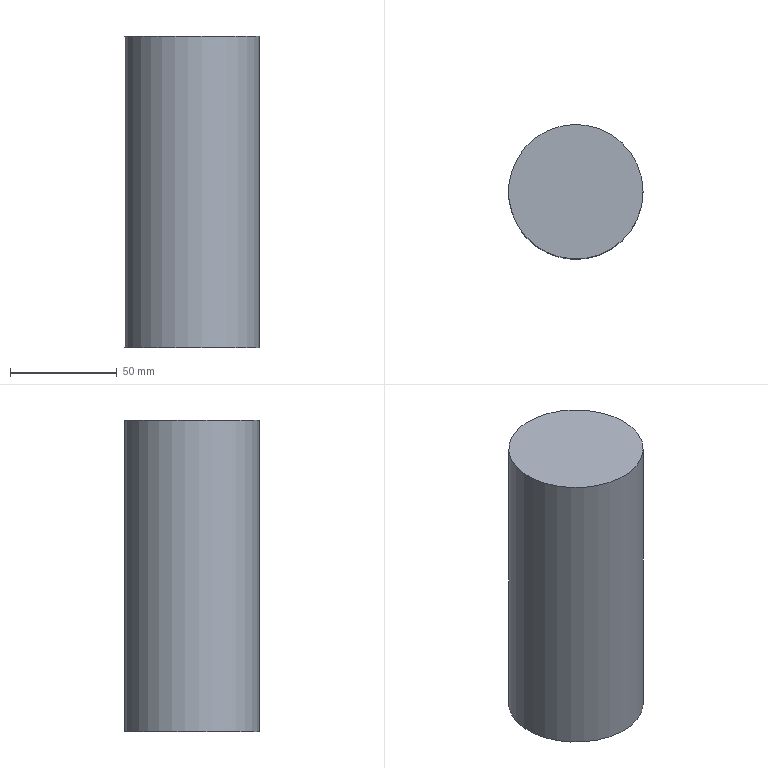Part | NX | features solid 2 | 1 solid | 3 faces | box 63 x 63 x 146 mm | volume 455118 mm3 | plane 2 | cylinder 1 | commonest cylinder face diameters 63 x1
STEP:
#1=CARTESIAN_POINT('',(31.5,-440.,-346.));
#2=VERTEX_POINT('',#1);
#3=CARTESIAN_POINT('',(0.,-440.,-346.));
#4=DIRECTION('',(0.,0.,1.));
#5=DIRECTION('',(1.,0.,0.));
#6=AXIS2_PLACEMENT_3D('',#3,#4,#5);
#7=CIRCLE('',#6,31.5);
#8=EDGE_CURVE('',#2,#2,#7,.T.);
#9=ORIENTED_EDGE('',*,*,#8,.T.);
#10=EDGE_LOOP('',(#9));
#11=FACE_BOUND('',#10,.T.);
#12=CARTESIAN_POINT('',(31.5,-440.,-200.));
#13=VERTEX_POINT('',#12);
#14=CARTESIAN_POINT('',(0.,-440.,-200.));
#15=DIRECTION('',(0.,0.,1.));
#16=DIRECTION('',(1.,0.,0.));
#17=AXIS2_PLACEMENT_3D('',#14,#15,#16);
#18=CIRCLE('',#17,31.5);
#19=EDGE_CURVE('',#13,#13,#18,.T.);
#20=ORIENTED_EDGE('',*,*,#19,.F.);
#21=EDGE_LOOP('',(#20));
#22=FACE_BOUND('',#21,.T.);
#23=CARTESIAN_POINT('',(0.,-440.,-476.));
#24=DIRECTION('',(0.,0.,1.));
#25=DIRECTION('',(-1.,0.,0.));
#26=AXIS2_PLACEMENT_3D('',#23,#24,#25);
#27=CYLINDRICAL_SURFACE('',#26,31.5);
#28=ADVANCED_FACE('',(#11,#22),#27,.T.);
#29=ORIENTED_EDGE('',*,*,#8,.F.);
#30=EDGE_LOOP('',(#29));
#31=FACE_BOUND('',#30,.T.);
#32=CARTESIAN_POINT('',(-35.,-475.,-346.));
#33=DIRECTION('',(0.,0.,-1.));
#34=DIRECTION('',(1.,0.,0.));
#35=AXIS2_PLACEMENT_3D('',#32,#33,#34);
#36=PLANE('',#35);
#37=ADVANCED_FACE('',(#31),#36,.T.);
#38=ORIENTED_EDGE('',*,*,#19,.T.);
#39=EDGE_LOOP('',(#38));
#40=FACE_BOUND('',#39,.T.);
#41=CARTESIAN_POINT('',(0.,-440.,-200.));
#42=DIRECTION('',(0.,0.,-1.));
#43=DIRECTION('',(1.,0.,0.));
#44=AXIS2_PLACEMENT_3D('',#41,#42,#43);
#45=PLANE('',#44);
#46=ADVANCED_FACE('',(#40),#45,.F.);
#47=CLOSED_SHELL('',(#28,#37,#46));
#48=MANIFOLD_SOLID_BREP('',#47);
#49=(LENGTH_UNIT()NAMED_UNIT(*)SI_UNIT(.MILLI.,.METRE.));
#50=UNCERTAINTY_MEASURE_WITH_UNIT(LENGTH_MEASURE(0.00001),#49,'','');
#51=(NAMED_UNIT(*)PLANE_ANGLE_UNIT()SI_UNIT($,.RADIAN.));
#52=(NAMED_UNIT(*)SI_UNIT($,.STERADIAN.)SOLID_ANGLE_UNIT());
#53=(GEOMETRIC_REPRESENTATION_CONTEXT(3)GLOBAL_UNCERTAINTY_ASSIGNED_CONTEXT((#50))GLOBAL_UNIT_ASSIGNED_CONTEXT((#49,#51,#52))REPRESENTATION_CONTEXT('',''));
#54=ADVANCED_BREP_SHAPE_REPRESENTATION('',(#48),#53);